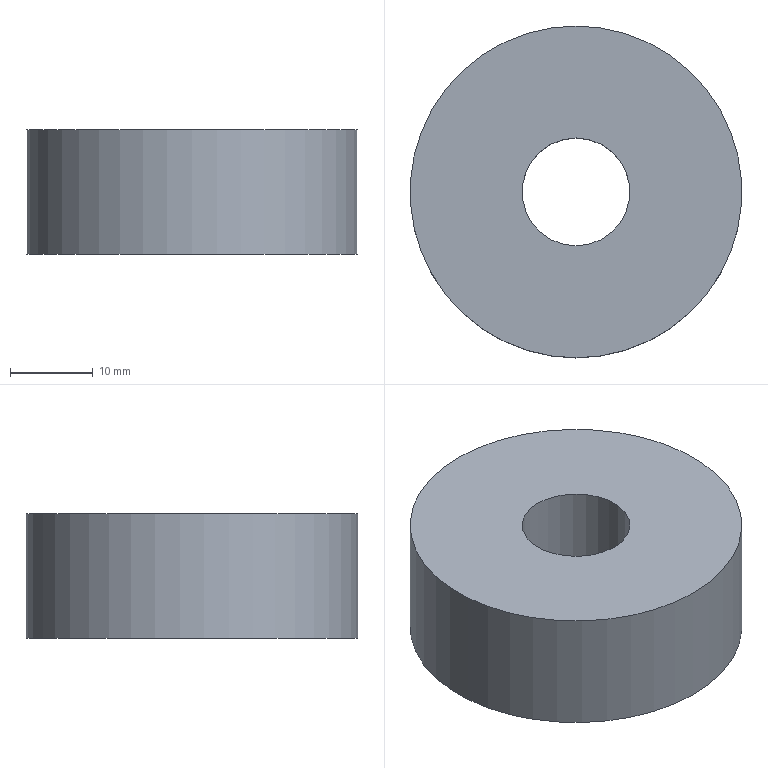Part | NX | features solid 2 | 1 solid | 4 faces | box 40 x 40 x 15 mm | volume 16859 mm3 | cylinder 2 | plane 2 | commonest cylinder face diameters 13 x1 40 x1
STEP:
#1=CARTESIAN_POINT('',(195.,45.,195.));
#2=VERTEX_POINT('',#1);
#3=CARTESIAN_POINT('',(195.,25.,195.));
#4=DIRECTION('',(0.000000001,-0.000000001,-1.));
#5=DIRECTION('',(0.,1.,-0.000000001));
#6=AXIS2_PLACEMENT_3D('',#3,#4,#5);
#7=CIRCLE('',#6,20.);
#8=EDGE_CURVE('',#2,#2,#7,.T.);
#9=ORIENTED_EDGE('',*,*,#8,.F.);
#10=EDGE_LOOP('',(#9));
#11=FACE_BOUND('',#10,.T.);
#12=CARTESIAN_POINT('',(195.,45.,210.));
#13=VERTEX_POINT('',#12);
#14=CARTESIAN_POINT('',(195.,25.,210.));
#15=DIRECTION('',(0.000000001,-0.000000001,-1.));
#16=DIRECTION('',(0.,1.,-0.000000001));
#17=AXIS2_PLACEMENT_3D('',#14,#15,#16);
#18=CIRCLE('',#17,20.);
#19=EDGE_CURVE('',#13,#13,#18,.T.);
#20=ORIENTED_EDGE('',*,*,#19,.T.);
#21=EDGE_LOOP('',(#20));
#22=FACE_BOUND('',#21,.T.);
#23=CARTESIAN_POINT('',(195.,25.,195.));
#24=DIRECTION('',(0.,0.,1.));
#25=DIRECTION('',(1.,0.,0.));
#26=AXIS2_PLACEMENT_3D('',#23,#24,#25);
#27=CYLINDRICAL_SURFACE('',#26,20.);
#28=ADVANCED_FACE('',(#11,#22),#27,.T.);
#29=CARTESIAN_POINT('',(195.,31.5,195.));
#30=VERTEX_POINT('',#29);
#31=CARTESIAN_POINT('',(195.,25.,195.));
#32=DIRECTION('',(0.000000001,-0.000000001,-1.));
#33=DIRECTION('',(0.,1.,-0.000000001));
#34=AXIS2_PLACEMENT_3D('',#31,#32,#33);
#35=CIRCLE('',#34,6.5);
#36=EDGE_CURVE('',#30,#30,#35,.T.);
#37=ORIENTED_EDGE('',*,*,#36,.F.);
#38=EDGE_LOOP('',(#37));
#39=FACE_BOUND('',#38,.T.);
#40=ORIENTED_EDGE('',*,*,#8,.T.);
#41=EDGE_LOOP('',(#40));
#42=FACE_BOUND('',#41,.T.);
#43=CARTESIAN_POINT('',(195.,25.,195.));
#44=DIRECTION('',(0.000000001,-0.000000001,-1.));
#45=DIRECTION('',(0.,1.,-0.000000001));
#46=AXIS2_PLACEMENT_3D('',#43,#44,#45);
#47=PLANE('',#46);
#48=ADVANCED_FACE('',(#39,#42),#47,.T.);
#49=ORIENTED_EDGE('',*,*,#19,.F.);
#50=EDGE_LOOP('',(#49));
#51=FACE_BOUND('',#50,.T.);
#52=CARTESIAN_POINT('',(195.,31.5,210.));
#53=VERTEX_POINT('',#52);
#54=CARTESIAN_POINT('',(195.,25.,210.));
#55=DIRECTION('',(0.000000001,-0.000000001,-1.));
#56=DIRECTION('',(0.,1.,-0.000000001));
#57=AXIS2_PLACEMENT_3D('',#54,#55,#56);
#58=CIRCLE('',#57,6.5);
#59=EDGE_CURVE('',#53,#53,#58,.F.);
#60=ORIENTED_EDGE('',*,*,#59,.F.);
#61=EDGE_LOOP('',(#60));
#62=FACE_BOUND('',#61,.T.);
#63=CARTESIAN_POINT('',(419.759,141.176,210.));
#64=DIRECTION('',(0.000000001,-0.000000001,-1.));
#65=DIRECTION('',(0.,1.,-0.000000001));
#66=AXIS2_PLACEMENT_3D('',#63,#64,#65);
#67=PLANE('',#66);
#68=ADVANCED_FACE('',(#51,#62),#67,.F.);
#69=ORIENTED_EDGE('',*,*,#36,.T.);
#70=EDGE_LOOP('',(#69));
#71=FACE_BOUND('',#70,.T.);
#72=ORIENTED_EDGE('',*,*,#59,.T.);
#73=EDGE_LOOP('',(#72));
#74=FACE_BOUND('',#73,.T.);
#75=CARTESIAN_POINT('',(195.,25.,215.));
#76=DIRECTION('',(0.,0.,-1.));
#77=DIRECTION('',(1.,0.,0.));
#78=AXIS2_PLACEMENT_3D('',#75,#76,#77);
#79=CYLINDRICAL_SURFACE('',#78,6.5);
#80=ADVANCED_FACE('',(#71,#74),#79,.F.);
#81=CLOSED_SHELL('',(#28,#48,#68,#80));
#82=MANIFOLD_SOLID_BREP('',#81);
#83=(LENGTH_UNIT()NAMED_UNIT(*)SI_UNIT(.MILLI.,.METRE.));
#84=UNCERTAINTY_MEASURE_WITH_UNIT(LENGTH_MEASURE(0.00001),#83,'','');
#85=(NAMED_UNIT(*)PLANE_ANGLE_UNIT()SI_UNIT($,.RADIAN.));
#86=(NAMED_UNIT(*)SI_UNIT($,.STERADIAN.)SOLID_ANGLE_UNIT());
#87=(GEOMETRIC_REPRESENTATION_CONTEXT(3)GLOBAL_UNCERTAINTY_ASSIGNED_CONTEXT((#84))GLOBAL_UNIT_ASSIGNED_CONTEXT((#83,#85,#86))REPRESENTATION_CONTEXT('',''));
#88=ADVANCED_BREP_SHAPE_REPRESENTATION('',(#82),#87);